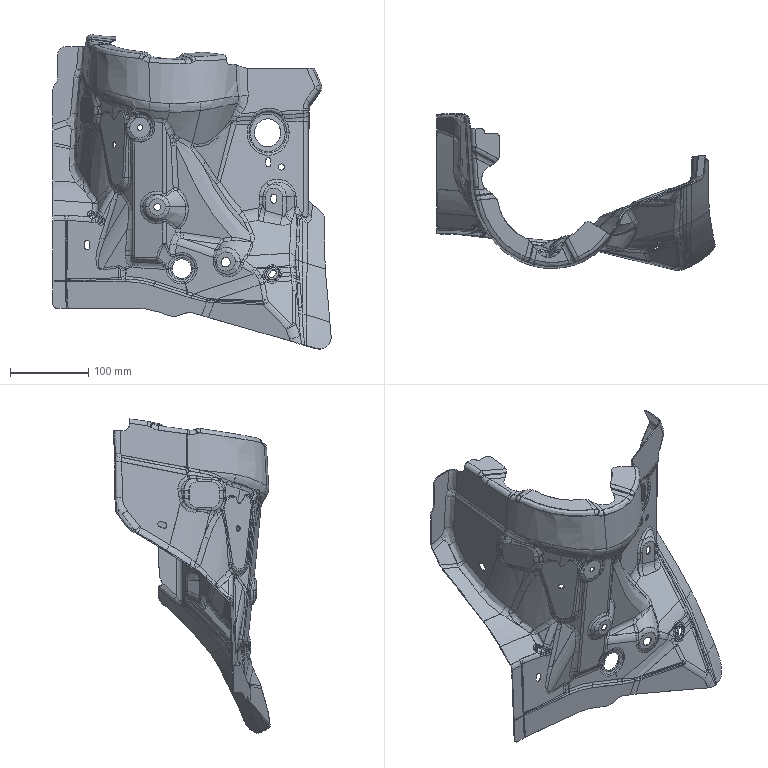Part | 1 solid | 1405 faces | box 355.591 x 199.989 x 401.521 mm | volume 194769 mm3 | spline 1070 | cylinder 196 | plane 112 | sphere 22 | other 5 | commonest cylinder face diameters 10 x18 20 x16 7.6 x15 7 x14 24 x13 17.6 x10